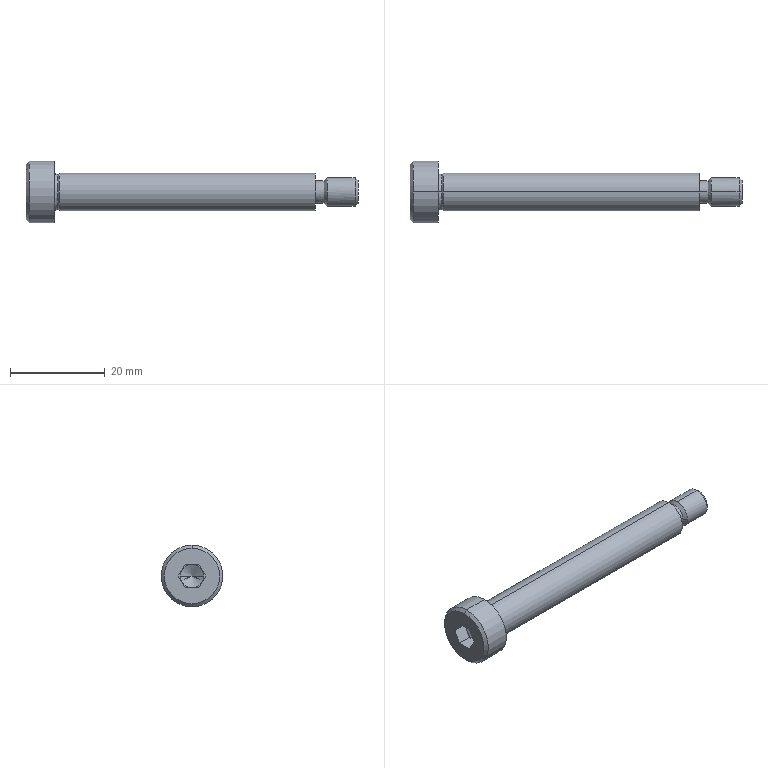Part | SolidWorks | features BaseBody 1 | 1 solid | 36 faces | box 70 x 13 x 13 mm | volume 3701 mm3 | plane 16 | cone 10 | cylinder 8 | spline 2 | commonest cylinder face diameters 4.7 x2 6 x2 8 x2 13 x2
STEP:
#1=CARTESIAN_POINT('',(0.,0.,4.35));
#2=VERTEX_POINT('',#1);
#3=CARTESIAN_POINT('',(0.,0.,-4.35));
#4=VERTEX_POINT('',#3);
#5=CARTESIAN_POINT('',(0.,0.,4.35));
#6=CARTESIAN_POINT('',(0.,0.2768,4.35));
#7=CARTESIAN_POINT('',(0.,0.6845,4.312));
#8=CARTESIAN_POINT('',(0.,1.147,4.2));
#9=CARTESIAN_POINT('',(0.,1.375,4.128));
#10=CARTESIAN_POINT('',(0.,1.472,4.093));
#11=CARTESIAN_POINT('',(0.,1.537,4.07));
#12=CARTESIAN_POINT('',(0.,1.567,4.058));
#13=CARTESIAN_POINT('',(0.,1.738,3.99));
#14=CARTESIAN_POINT('',(0.,1.938,3.899));
#15=CARTESIAN_POINT('',(0.,2.13,3.793));
#16=CARTESIAN_POINT('',(0.,2.257,3.72));
#17=CARTESIAN_POINT('',(0.,2.317,3.682));
#18=CARTESIAN_POINT('',(0.,2.632,3.476));
#19=CARTESIAN_POINT('',(0.,2.863,3.289));
#20=CARTESIAN_POINT('',(0.,3.182,2.97));
#21=CARTESIAN_POINT('',(0.,3.333,2.803));
#22=CARTESIAN_POINT('',(0.,3.469,2.625));
#23=CARTESIAN_POINT('',(0.,3.557,2.505));
#24=CARTESIAN_POINT('',(0.,3.601,2.442));
#25=CARTESIAN_POINT('',(0.,3.721,2.257));
#26=CARTESIAN_POINT('',(0.,3.832,2.067));
#27=CARTESIAN_POINT('',(0.,3.944,1.837));
#28=CARTESIAN_POINT('',(0.,3.988,1.737));
#29=CARTESIAN_POINT('',(0.,4.017,1.669));
#30=CARTESIAN_POINT('',(0.,4.032,1.633));
#31=CARTESIAN_POINT('',(0.,4.248,1.087));
#32=CARTESIAN_POINT('',(0.,4.35,0.5535));
#33=CARTESIAN_POINT('',(0.,4.35,-0.2768));
#34=CARTESIAN_POINT('',(0.,4.312,-0.6845));
#35=CARTESIAN_POINT('',(0.,4.2,-1.147));
#36=CARTESIAN_POINT('',(0.,4.128,-1.375));
#37=CARTESIAN_POINT('',(0.,4.093,-1.472));
#38=CARTESIAN_POINT('',(0.,4.07,-1.537));
#39=CARTESIAN_POINT('',(0.,4.058,-1.567));
#40=CARTESIAN_POINT('',(0.,3.99,-1.738));
#41=CARTESIAN_POINT('',(0.,3.899,-1.938));
#42=CARTESIAN_POINT('',(0.,3.793,-2.13));
#43=CARTESIAN_POINT('',(0.,3.72,-2.257));
#44=CARTESIAN_POINT('',(0.,3.682,-2.317));
#45=CARTESIAN_POINT('',(0.,3.476,-2.632));
#46=CARTESIAN_POINT('',(0.,3.289,-2.863));
#47=CARTESIAN_POINT('',(0.,2.97,-3.182));
#48=CARTESIAN_POINT('',(0.,2.803,-3.333));
#49=CARTESIAN_POINT('',(0.,2.625,-3.469));
#50=CARTESIAN_POINT('',(0.,2.505,-3.557));
#51=CARTESIAN_POINT('',(0.,2.442,-3.601));
#52=CARTESIAN_POINT('',(0.,2.257,-3.721));
#53=CARTESIAN_POINT('',(0.,2.067,-3.832));
#54=CARTESIAN_POINT('',(0.,1.837,-3.944));
#55=CARTESIAN_POINT('',(0.,1.737,-3.988));
#56=CARTESIAN_POINT('',(0.,1.669,-4.017));
#57=CARTESIAN_POINT('',(0.,1.633,-4.032));
#58=CARTESIAN_POINT('',(0.,1.087,-4.248));
#59=CARTESIAN_POINT('',(0.,0.553,-4.35));
#60=CARTESIAN_POINT('',(0.,0.,-4.35));
#61=B_SPLINE_CURVE_WITH_KNOTS('',3,(#5,#6,#7,#8,#9,#10,#11,#12,#13,#14,#15,#16,#17,#18,#19,#20,#21,#22,#23,#24,#25,#26,#27,#28,#29,#30,#31,#32,#33,#34,#35,#36,#37,#38,#39,#40,#41,#42,#43,#44,#45,#46,#47,#48,#49,#50,#51,#52,#53,#54,#55,#56,#57,#58,#59,#60),.UNSPECIFIED.,.F.,.F.,(4,1,1,1,2,2,1,2,2,2,1,2,2,1,1,2,2,2,1,1,1,2,2,1,2,2,2,1,2,2,1,1,2,2,4),(0.5,0.5313,0.5469,0.5547,0.5586,0.5625,0.5781,0.5859,0.5938,0.625,0.6406,0.6484,0.6563,0.6719,0.6797,0.6836,0.6875,0.75,0.7813,0.7969,0.8047,0.8086,0.8125,0.8281,0.8359,0.8438,0.875,0.8906,0.8984,0.9063,0.9219,0.9297,0.9336,0.9375,1.),.UNSPECIFIED.);
#62=EDGE_CURVE('',#2,#4,#61,.T.);
#63=ORIENTED_EDGE('',*,*,#62,.F.);
#64=CARTESIAN_POINT('',(0.7,0.,3.7));
#65=VERTEX_POINT('',#64);
#66=CARTESIAN_POINT('',(0.6306,0.,4.327));
#67=DIRECTION('',(0.,-1.,0.));
#68=DIRECTION('',(0.,0.,1.));
#69=AXIS2_PLACEMENT_3D('',#66,#67,#68);
#70=CIRCLE('',#69,0.631);
#71=EDGE_CURVE('',#2,#65,#70,.T.);
#72=ORIENTED_EDGE('',*,*,#71,.T.);
#73=CARTESIAN_POINT('',(0.7,0.,-3.7));
#74=VERTEX_POINT('',#73);
#75=CARTESIAN_POINT('',(0.7,0.,0.));
#76=DIRECTION('',(1.,0.,0.));
#77=DIRECTION('',(0.,0.,-1.));
#78=AXIS2_PLACEMENT_3D('',#75,#76,#77);
#79=CIRCLE('',#78,3.7);
#80=EDGE_CURVE('',#74,#65,#79,.T.);
#81=ORIENTED_EDGE('',*,*,#80,.F.);
#82=CARTESIAN_POINT('',(0.6306,0.,-4.327));
#83=DIRECTION('',(0.,1.,0.));
#84=DIRECTION('',(0.,0.,-1.));
#85=AXIS2_PLACEMENT_3D('',#82,#83,#84);
#86=CIRCLE('',#85,0.631);
#87=EDGE_CURVE('',#4,#74,#86,.T.);
#88=ORIENTED_EDGE('',*,*,#87,.F.);
#89=EDGE_LOOP('',(#63,#72,#81,#88));
#90=FACE_OUTER_BOUND('',#89,.T.);
#91=CARTESIAN_POINT('',(0.,0.,-4.35));
#92=CARTESIAN_POINT('',(0.,8.7,-4.35));
#93=CARTESIAN_POINT('',(0.,8.7,4.35));
#94=CARTESIAN_POINT('',(0.,0.,4.35));
#95=CARTESIAN_POINT('',(-0.01498,0.,-3.936));
#96=CARTESIAN_POINT('',(-0.01498,7.872,-3.936));
#97=CARTESIAN_POINT('',(-0.01498,7.872,3.936));
#98=CARTESIAN_POINT('',(-0.01498,0.,3.936));
#99=CARTESIAN_POINT('',(0.2884,0.,-3.654));
#100=CARTESIAN_POINT('',(0.2884,7.309,-3.654));
#101=CARTESIAN_POINT('',(0.2884,7.309,3.654));
#102=CARTESIAN_POINT('',(0.2884,0.,3.654));
#103=CARTESIAN_POINT('',(0.7,0.,-3.7));
#104=CARTESIAN_POINT('',(0.7,7.4,-3.7));
#105=CARTESIAN_POINT('',(0.7,7.4,3.7));
#106=CARTESIAN_POINT('',(0.7,0.,3.7));
#107=(BOUNDED_SURFACE()B_SPLINE_SURFACE(3,3,((#91,#92,#93,#94),(#95,#96,#97,#98),(#99,#100,#101,#102),(#103,#104,#105,#106)),.UNSPECIFIED.,.F.,.F.,.T.)B_SPLINE_SURFACE_WITH_KNOTS((4,4),(4,4),(0.,1.),(0.,1.),.UNSPECIFIED.)GEOMETRIC_REPRESENTATION_ITEM()RATIONAL_B_SPLINE_SURFACE(((1.,0.3333,0.3333,1.),(0.769,0.2563,0.2563,0.769),(0.769,0.2563,0.2563,0.769),(1.,0.3333,0.3333,1.)))REPRESENTATION_ITEM('')SURFACE());
#108=ADVANCED_FACE('',(#90),#107,.F.);
#109=CARTESIAN_POINT('',(55.,0.,4.));
#110=VERTEX_POINT('',#109);
#111=CARTESIAN_POINT('',(55.,0.,-4.));
#112=VERTEX_POINT('',#111);
#113=CARTESIAN_POINT('',(55.,0.,0.));
#114=DIRECTION('',(-1.,0.,0.));
#115=DIRECTION('',(0.,0.,1.));
#116=AXIS2_PLACEMENT_3D('',#113,#114,#115);
#117=CIRCLE('',#116,4.);
#118=EDGE_CURVE('',#110,#112,#117,.T.);
#119=ORIENTED_EDGE('',*,*,#118,.T.);
#120=CARTESIAN_POINT('',(1.,0.,-4.));
#121=VERTEX_POINT('',#120);
#122=CARTESIAN_POINT('',(64.,0.,-4.));
#123=DIRECTION('',(-1.,0.,0.));
#124=VECTOR('',#123,1000.);
#125=LINE('',#122,#124);
#126=EDGE_CURVE('',#112,#121,#125,.T.);
#127=ORIENTED_EDGE('',*,*,#126,.T.);
#128=CARTESIAN_POINT('',(1.,0.,4.));
#129=VERTEX_POINT('',#128);
#130=CARTESIAN_POINT('',(1.,0.,0.));
#131=DIRECTION('',(1.,0.,0.));
#132=DIRECTION('',(0.,0.,1.));
#133=AXIS2_PLACEMENT_3D('',#130,#131,#132);
#134=CIRCLE('',#133,4.);
#135=EDGE_CURVE('',#121,#129,#134,.T.);
#136=ORIENTED_EDGE('',*,*,#135,.T.);
#137=CARTESIAN_POINT('',(64.,0.,4.));
#138=DIRECTION('',(-1.,0.,0.));
#139=VECTOR('',#138,1000.);
#140=LINE('',#137,#139);
#141=EDGE_CURVE('',#110,#129,#140,.T.);
#142=ORIENTED_EDGE('',*,*,#141,.F.);
#143=EDGE_LOOP('',(#119,#127,#136,#142));
#144=FACE_OUTER_BOUND('',#143,.T.);
#145=CARTESIAN_POINT('',(64.,0.,0.));
#146=DIRECTION('',(-1.,0.,0.));
#147=DIRECTION('',(0.,0.,1.));
#148=AXIS2_PLACEMENT_3D('',#145,#146,#147);
#149=CYLINDRICAL_SURFACE('',#148,4.);
#150=ADVANCED_FACE('',(#144),#149,.T.);
#151=ORIENTED_EDGE('',*,*,#80,.T.);
#152=CARTESIAN_POINT('',(1.,0.,4.));
#153=DIRECTION('',(0.7071,0.,0.7071));
#154=VECTOR('',#153,1000.);
#155=LINE('',#152,#154);
#156=EDGE_CURVE('',#65,#129,#155,.T.);
#157=ORIENTED_EDGE('',*,*,#156,.T.);
#158=ORIENTED_EDGE('',*,*,#135,.F.);
#159=CARTESIAN_POINT('',(1.,0.,-4.));
#160=DIRECTION('',(0.7071,0.,-0.7071));
#161=VECTOR('',#160,1000.);
#162=LINE('',#159,#161);
#163=EDGE_CURVE('',#74,#121,#162,.T.);
#164=ORIENTED_EDGE('',*,*,#163,.F.);
#165=EDGE_LOOP('',(#151,#157,#158,#164));
#166=FACE_OUTER_BOUND('',#165,.T.);
#167=CARTESIAN_POINT('',(1.,0.,0.));
#168=DIRECTION('',(1.,0.,0.));
#169=DIRECTION('',(0.,0.,-1.));
#170=AXIS2_PLACEMENT_3D('',#167,#168,#169);
#171=CONICAL_SURFACE('',#170,4.,0.7854);
#172=ADVANCED_FACE('',(#166),#171,.T.);
#173=CARTESIAN_POINT('',(56.85,2.35,0.));
#174=VERTEX_POINT('',#173);
#175=CARTESIAN_POINT('',(56.85,0.,-2.35));
#176=VERTEX_POINT('',#175);
#177=CARTESIAN_POINT('',(56.85,0.,0.));
#178=DIRECTION('',(-1.,0.,0.));
#179=DIRECTION('',(0.,0.,1.));
#180=AXIS2_PLACEMENT_3D('',#177,#178,#179);
#181=CIRCLE('',#180,2.35);
#182=EDGE_CURVE('',#174,#176,#181,.T.);
#183=ORIENTED_EDGE('',*,*,#182,.T.);
#184=CARTESIAN_POINT('',(55.,0.,-2.35));
#185=VERTEX_POINT('',#184);
#186=CARTESIAN_POINT('',(64.,0.,-2.35));
#187=DIRECTION('',(-1.,0.,0.));
#188=VECTOR('',#187,1000.);
#189=LINE('',#186,#188);
#190=EDGE_CURVE('',#176,#185,#189,.T.);
#191=ORIENTED_EDGE('',*,*,#190,.T.);
#192=CARTESIAN_POINT('',(55.,0.,2.35));
#193=VERTEX_POINT('',#192);
#194=CARTESIAN_POINT('',(55.,0.,0.));
#195=DIRECTION('',(1.,0.,0.));
#196=DIRECTION('',(0.,0.,1.));
#197=AXIS2_PLACEMENT_3D('',#194,#195,#196);
#198=CIRCLE('',#197,2.35);
#199=EDGE_CURVE('',#185,#193,#198,.T.);
#200=ORIENTED_EDGE('',*,*,#199,.T.);
#201=CARTESIAN_POINT('',(56.85,0.,2.35));
#202=VERTEX_POINT('',#201);
#203=CARTESIAN_POINT('',(64.,0.,2.35));
#204=DIRECTION('',(-1.,0.,0.));
#205=VECTOR('',#204,1000.);
#206=LINE('',#203,#205);
#207=EDGE_CURVE('',#202,#193,#206,.T.);
#208=ORIENTED_EDGE('',*,*,#207,.F.);
#209=CARTESIAN_POINT('',(56.85,0.,0.));
#210=DIRECTION('',(-1.,0.,0.));
#211=DIRECTION('',(0.,0.,1.));
#212=AXIS2_PLACEMENT_3D('',#209,#210,#211);
#213=CIRCLE('',#212,2.35);
#214=EDGE_CURVE('',#202,#174,#213,.T.);
#215=ORIENTED_EDGE('',*,*,#214,.T.);
#216=EDGE_LOOP('',(#183,#191,#200,#208,#215));
#217=FACE_OUTER_BOUND('',#216,.T.);
#218=CARTESIAN_POINT('',(64.,0.,0.));
#219=DIRECTION('',(-1.,0.,0.));
#220=DIRECTION('',(0.,0.,1.));
#221=AXIS2_PLACEMENT_3D('',#218,#219,#220);
#222=CYLINDRICAL_SURFACE('',#221,2.35);
#223=ADVANCED_FACE('',(#217),#222,.T.);
#224=CARTESIAN_POINT('',(56.85,-2.35,0.));
#225=VERTEX_POINT('',#224);
#226=CARTESIAN_POINT('',(56.85,0.,0.));
#227=DIRECTION('',(-1.,0.,0.));
#228=DIRECTION('',(0.,0.,1.));
#229=AXIS2_PLACEMENT_3D('',#226,#227,#228);
#230=CIRCLE('',#229,2.35);
#231=EDGE_CURVE('',#225,#202,#230,.T.);
#232=ORIENTED_EDGE('',*,*,#231,.F.);
#233=CARTESIAN_POINT('',(57.5,-3.,0.));
#234=VERTEX_POINT('',#233);
#235=CARTESIAN_POINT('',(57.5,-3.,0.));
#236=DIRECTION('',(0.7071,-0.7071,0.));
#237=VECTOR('',#236,1000.);
#238=LINE('',#235,#237);
#239=EDGE_CURVE('',#225,#234,#238,.T.);
#240=ORIENTED_EDGE('',*,*,#239,.T.);
#241=CARTESIAN_POINT('',(57.5,0.,3.));
#242=VERTEX_POINT('',#241);
#243=CARTESIAN_POINT('',(57.5,0.,0.));
#244=DIRECTION('',(-1.,0.,0.));
#245=DIRECTION('',(0.,0.,-1.));
#246=AXIS2_PLACEMENT_3D('',#243,#244,#245);
#247=CIRCLE('',#246,3.);
#248=EDGE_CURVE('',#234,#242,#247,.T.);
#249=ORIENTED_EDGE('',*,*,#248,.T.);
#250=CARTESIAN_POINT('',(57.5,3.,0.));
#251=VERTEX_POINT('',#250);
#252=CARTESIAN_POINT('',(57.5,0.,0.));
#253=DIRECTION('',(-1.,0.,0.));
#254=DIRECTION('',(0.,0.,-1.));
#255=AXIS2_PLACEMENT_3D('',#252,#253,#254);
#256=CIRCLE('',#255,3.);
#257=EDGE_CURVE('',#242,#251,#256,.T.);
#258=ORIENTED_EDGE('',*,*,#257,.T.);
#259=CARTESIAN_POINT('',(57.5,3.,0.));
#260=DIRECTION('',(0.7071,0.7071,0.));
#261=VECTOR('',#260,1000.);
#262=LINE('',#259,#261);
#263=EDGE_CURVE('',#174,#251,#262,.T.);
#264=ORIENTED_EDGE('',*,*,#263,.F.);
#265=ORIENTED_EDGE('',*,*,#214,.F.);
#266=EDGE_LOOP('',(#232,#240,#249,#258,#264,#265));
#267=FACE_OUTER_BOUND('',#266,.T.);
#268=CARTESIAN_POINT('',(57.5,0.,0.));
#269=DIRECTION('',(1.,0.,0.));
#270=DIRECTION('',(0.,1.,0.));
#271=AXIS2_PLACEMENT_3D('',#268,#269,#270);
#272=CONICAL_SURFACE('',#271,3.,0.7854);
#273=ADVANCED_FACE('',(#267),#272,.T.);
#274=CARTESIAN_POINT('',(0.,0.,6.5));
#275=VERTEX_POINT('',#274);
#276=CARTESIAN_POINT('',(0.,0.,-6.5));
#277=VERTEX_POINT('',#276);
#278=CARTESIAN_POINT('',(0.,0.,0.));
#279=DIRECTION('',(-1.,0.,0.));
#280=DIRECTION('',(0.,0.,1.));
#281=AXIS2_PLACEMENT_3D('',#278,#279,#280);
#282=CIRCLE('',#281,6.5);
#283=EDGE_CURVE('',#275,#277,#282,.T.);
#284=ORIENTED_EDGE('',*,*,#283,.T.);
#285=CARTESIAN_POINT('',(-5.35,0.,-6.5));
#286=VERTEX_POINT('',#285);
#287=CARTESIAN_POINT('',(64.,0.,-6.5));
#288=DIRECTION('',(-1.,0.,0.));
#289=VECTOR('',#288,1000.);
#290=LINE('',#287,#289);
#291=EDGE_CURVE('',#277,#286,#290,.T.);
#292=ORIENTED_EDGE('',*,*,#291,.T.);
#293=CARTESIAN_POINT('',(-5.35,0.,6.5));
#294=VERTEX_POINT('',#293);
#295=CARTESIAN_POINT('',(-5.35,0.,0.));
#296=DIRECTION('',(1.,0.,0.));
#297=DIRECTION('',(0.,0.,1.));
#298=AXIS2_PLACEMENT_3D('',#295,#296,#297);
#299=CIRCLE('',#298,6.5);
#300=EDGE_CURVE('',#286,#294,#299,.T.);
#301=ORIENTED_EDGE('',*,*,#300,.T.);
#302=CARTESIAN_POINT('',(64.,0.,6.5));
#303=DIRECTION('',(-1.,0.,0.));
#304=VECTOR('',#303,1000.);
#305=LINE('',#302,#304);
#306=EDGE_CURVE('',#275,#294,#305,.T.);
#307=ORIENTED_EDGE('',*,*,#306,.F.);
#308=EDGE_LOOP('',(#284,#292,#301,#307));
#309=FACE_OUTER_BOUND('',#308,.T.);
#310=CARTESIAN_POINT('',(64.,0.,0.));
#311=DIRECTION('',(-1.,0.,0.));
#312=DIRECTION('',(0.,0.,1.));
#313=AXIS2_PLACEMENT_3D('',#310,#311,#312);
#314=CYLINDRICAL_SURFACE('',#313,6.5);
#315=ADVANCED_FACE('',(#309),#314,.T.);
#316=CARTESIAN_POINT('',(63.386,0.,3.));
#317=VERTEX_POINT('',#316);
#318=CARTESIAN_POINT('',(63.386,0.,-3.));
#319=VERTEX_POINT('',#318);
#320=CARTESIAN_POINT('',(63.386,0.,0.));
#321=DIRECTION('',(-1.,0.,0.));
#322=DIRECTION('',(0.,0.,1.));
#323=AXIS2_PLACEMENT_3D('',#320,#321,#322);
#324=CIRCLE('',#323,3.);
#325=EDGE_CURVE('',#317,#319,#324,.T.);
#326=ORIENTED_EDGE('',*,*,#325,.T.);
#327=CARTESIAN_POINT('',(57.5,0.,-3.));
#328=VERTEX_POINT('',#327);
#329=CARTESIAN_POINT('',(64.,0.,-3.));
#330=DIRECTION('',(-1.,0.,0.));
#331=VECTOR('',#330,1000.);
#332=LINE('',#329,#331);
#333=EDGE_CURVE('',#319,#328,#332,.T.);
#334=ORIENTED_EDGE('',*,*,#333,.T.);
#335=CARTESIAN_POINT('',(57.5,0.,0.));
#336=DIRECTION('',(-1.,0.,0.));
#337=DIRECTION('',(0.,0.,-1.));
#338=AXIS2_PLACEMENT_3D('',#335,#336,#337);
#339=CIRCLE('',#338,3.);
#340=EDGE_CURVE('',#251,#328,#339,.T.);
#341=ORIENTED_EDGE('',*,*,#340,.F.);
#342=ORIENTED_EDGE('',*,*,#257,.F.);
#343=CARTESIAN_POINT('',(64.,0.,3.));
#344=DIRECTION('',(-1.,0.,0.));
#345=VECTOR('',#344,1000.);
#346=LINE('',#343,#345);
#347=EDGE_CURVE('',#317,#242,#346,.T.);
#348=ORIENTED_EDGE('',*,*,#347,.F.);
#349=EDGE_LOOP('',(#326,#334,#341,#342,#348));
#350=FACE_OUTER_BOUND('',#349,.T.);
#351=CARTESIAN_POINT('',(64.,0.,0.));
#352=DIRECTION('',(-1.,0.,0.));
#353=DIRECTION('',(0.,0.,1.));
#354=AXIS2_PLACEMENT_3D('',#351,#352,#353);
#355=CYLINDRICAL_SURFACE('',#354,3.);
#356=ADVANCED_FACE('',(#350),#355,.T.);
#357=CARTESIAN_POINT('',(-6.,0.,-5.85));
#358=VERTEX_POINT('',#357);
#359=CARTESIAN_POINT('',(-6.,0.,5.85));
#360=VERTEX_POINT('',#359);
#361=CARTESIAN_POINT('',(-6.,0.,0.));
#362=DIRECTION('',(1.,0.,0.));
#363=DIRECTION('',(0.,0.,-1.));
#364=AXIS2_PLACEMENT_3D('',#361,#362,#363);
#365=CIRCLE('',#364,5.85);
#366=EDGE_CURVE('',#358,#360,#365,.T.);
#367=ORIENTED_EDGE('',*,*,#366,.T.);
#368=CARTESIAN_POINT('',(-5.35,0.,6.5));
#369=DIRECTION('',(0.7071,0.,0.7071));
#370=VECTOR('',#369,1000.);
#371=LINE('',#368,#370);
#372=EDGE_CURVE('',#360,#294,#371,.T.);
#373=ORIENTED_EDGE('',*,*,#372,.T.);
#374=ORIENTED_EDGE('',*,*,#300,.F.);
#375=CARTESIAN_POINT('',(-5.35,0.,-6.5));
#376=DIRECTION('',(0.7071,0.,-0.7071));
#377=VECTOR('',#376,1000.);
#378=LINE('',#375,#377);
#379=EDGE_CURVE('',#358,#286,#378,.T.);
#380=ORIENTED_EDGE('',*,*,#379,.F.);
#381=EDGE_LOOP('',(#367,#373,#374,#380));
#382=FACE_OUTER_BOUND('',#381,.T.);
#383=CARTESIAN_POINT('',(-5.35,0.,0.));
#384=DIRECTION('',(1.,0.,0.));
#385=DIRECTION('',(0.,0.,-1.));
#386=AXIS2_PLACEMENT_3D('',#383,#384,#385);
#387=CONICAL_SURFACE('',#386,6.5,0.7854);
#388=ADVANCED_FACE('',(#382),#387,.T.);
#389=CARTESIAN_POINT('',(64.,0.,2.386));
#390=VERTEX_POINT('',#389);
#391=CARTESIAN_POINT('',(64.,0.,-2.386));
#392=VERTEX_POINT('',#391);
#393=CARTESIAN_POINT('',(64.,0.,0.));
#394=DIRECTION('',(-1.,0.,0.));
#395=DIRECTION('',(0.,0.,1.));
#396=AXIS2_PLACEMENT_3D('',#393,#394,#395);
#397=CIRCLE('',#396,2.386);
#398=EDGE_CURVE('',#390,#392,#397,.T.);
#399=ORIENTED_EDGE('',*,*,#398,.T.);
#400=CARTESIAN_POINT('',(63.387,0.,-3.));
#401=DIRECTION('',(-0.7071,0.,-0.7071));
#402=VECTOR('',#401,1000.);
#403=LINE('',#400,#402);
#404=EDGE_CURVE('',#392,#319,#403,.T.);
#405=ORIENTED_EDGE('',*,*,#404,.T.);
#406=ORIENTED_EDGE('',*,*,#325,.F.);
#407=CARTESIAN_POINT('',(63.387,0.,3.));
#408=DIRECTION('',(-0.7071,0.,0.7071));
#409=VECTOR('',#408,1000.);
#410=LINE('',#407,#409);
#411=EDGE_CURVE('',#390,#317,#410,.T.);
#412=ORIENTED_EDGE('',*,*,#411,.F.);
#413=EDGE_LOOP('',(#399,#405,#406,#412));
#414=FACE_OUTER_BOUND('',#413,.T.);
#415=CARTESIAN_POINT('',(63.387,0.,0.));
#416=DIRECTION('',(-1.,0.,0.));
#417=DIRECTION('',(0.,0.,1.));
#418=AXIS2_PLACEMENT_3D('',#415,#416,#417);
#419=CONICAL_SURFACE('',#418,3.,0.7854);
#420=ADVANCED_FACE('',(#414),#419,.T.);
#421=CARTESIAN_POINT('',(-1.557,0.,0.));
#422=VERTEX_POINT('',#421);
#423=CARTESIAN_POINT('',(-3.,-2.5,0.));
#424=VERTEX_POINT('',#423);
#425=CARTESIAN_POINT('',(-3.,-2.5,0.));
#426=DIRECTION('',(-0.5,-0.866,0.));
#427=VECTOR('',#426,1000.);
#428=LINE('',#425,#427);
#429=EDGE_CURVE('',#422,#424,#428,.T.);
#430=ORIENTED_EDGE('',*,*,#429,.F.);
#431=CARTESIAN_POINT('',(-3.,2.5,0.));
#432=VERTEX_POINT('',#431);
#433=CARTESIAN_POINT('',(-3.,2.5,0.));
#434=DIRECTION('',(-0.5,0.866,0.));
#435=VECTOR('',#434,1000.);
#436=LINE('',#433,#435);
#437=EDGE_CURVE('',#422,#432,#436,.T.);
#438=ORIENTED_EDGE('',*,*,#437,.T.);
#439=CARTESIAN_POINT('',(-3.,2.165,-1.25));
#440=VERTEX_POINT('',#439);
#441=CARTESIAN_POINT('',(-3.,0.,0.));
#442=DIRECTION('',(1.,0.,0.));
#443=DIRECTION('',(0.,-1.,0.));
#444=AXIS2_PLACEMENT_3D('',#441,#442,#443);
#445=CIRCLE('',#444,2.5);
#446=EDGE_CURVE('',#440,#432,#445,.T.);
#447=ORIENTED_EDGE('',*,*,#446,.F.);
#448=CARTESIAN_POINT('',(-3.,0.,-2.5));
#449=VERTEX_POINT('',#448);
#450=CARTESIAN_POINT('',(-3.,0.,0.));
#451=DIRECTION('',(1.,0.,0.));
#452=DIRECTION('',(0.,-1.,0.));
#453=AXIS2_PLACEMENT_3D('',#450,#451,#452);
#454=CIRCLE('',#453,2.5);
#455=EDGE_CURVE('',#449,#440,#454,.T.);
#456=ORIENTED_EDGE('',*,*,#455,.F.);
#457=CARTESIAN_POINT('',(-3.,-2.165,-1.25));
#458=VERTEX_POINT('',#457);
#459=CARTESIAN_POINT('',(-3.,0.,0.));
#460=DIRECTION('',(1.,0.,0.));
#461=DIRECTION('',(0.,-1.,0.));
#462=AXIS2_PLACEMENT_3D('',#459,#460,#461);
#463=CIRCLE('',#462,2.5);
#464=EDGE_CURVE('',#458,#449,#463,.T.);
#465=ORIENTED_EDGE('',*,*,#464,.F.);
#466=CARTESIAN_POINT('',(-3.,0.,0.));
#467=DIRECTION('',(1.,0.,0.));
#468=DIRECTION('',(0.,-1.,0.));
#469=AXIS2_PLACEMENT_3D('',#466,#467,#468);
#470=CIRCLE('',#469,2.5);
#471=EDGE_CURVE('',#424,#458,#470,.T.);
#472=ORIENTED_EDGE('',*,*,#471,.F.);
#473=EDGE_LOOP('',(#430,#438,#447,#456,#465,#472));
#474=FACE_OUTER_BOUND('',#473,.T.);
#475=CARTESIAN_POINT('',(-3.,0.,0.));
#476=DIRECTION('',(-1.,0.,0.));
#477=DIRECTION('',(0.,-1.,0.));
#478=AXIS2_PLACEMENT_3D('',#475,#476,#477);
#479=CONICAL_SURFACE('',#478,2.5,1.047);
#480=ADVANCED_FACE('',(#474),#479,.F.);
#481=ORIENTED_EDGE('',*,*,#126,.F.);
#482=CARTESIAN_POINT('',(55.,0.,0.));
#483=DIRECTION('',(-1.,0.,0.));
#484=DIRECTION('',(0.,0.,1.));
#485=AXIS2_PLACEMENT_3D('',#482,#483,#484);
#486=CIRCLE('',#485,4.);
#487=EDGE_CURVE('',#112,#110,#486,.T.);
#488=ORIENTED_EDGE('',*,*,#487,.T.);
#489=ORIENTED_EDGE('',*,*,#141,.T.);
#490=CARTESIAN_POINT('',(1.,0.,0.));
#491=DIRECTION('',(1.,0.,0.));
#492=DIRECTION('',(0.,0.,1.));
#493=AXIS2_PLACEMENT_3D('',#490,#491,#492);
#494=CIRCLE('',#493,4.);
#495=EDGE_CURVE('',#129,#121,#494,.T.);
#496=ORIENTED_EDGE('',*,*,#495,.T.);
#497=EDGE_LOOP('',(#481,#488,#489,#496));
#498=FACE_OUTER_BOUND('',#497,.T.);
#499=CARTESIAN_POINT('',(64.,0.,0.));
#500=DIRECTION('',(-1.,0.,0.));
#501=DIRECTION('',(0.,0.,1.));
#502=AXIS2_PLACEMENT_3D('',#499,#500,#501);
#503=CYLINDRICAL_SURFACE('',#502,4.);
#504=ADVANCED_FACE('',(#498),#503,.T.);
#505=ORIENTED_EDGE('',*,*,#156,.F.);
#506=CARTESIAN_POINT('',(0.7,0.,0.));
#507=DIRECTION('',(1.,0.,0.));
#508=DIRECTION('',(0.,0.,-1.));
#509=AXIS2_PLACEMENT_3D('',#506,#507,#508);
#510=CIRCLE('',#509,3.7);
#511=EDGE_CURVE('',#65,#74,#510,.T.);
#512=ORIENTED_EDGE('',*,*,#511,.T.);
#513=ORIENTED_EDGE('',*,*,#163,.T.);
#514=ORIENTED_EDGE('',*,*,#495,.F.);
#515=EDGE_LOOP('',(#505,#512,#513,#514));
#516=FACE_OUTER_BOUND('',#515,.T.);
#517=CARTESIAN_POINT('',(1.,0.,0.));
#518=DIRECTION('',(1.,0.,0.));
#519=DIRECTION('',(0.,0.,-1.));
#520=AXIS2_PLACEMENT_3D('',#517,#518,#519);
#521=CONICAL_SURFACE('',#520,4.,0.7854);
#522=ADVANCED_FACE('',(#516),#521,.T.);
#523=ORIENTED_EDGE('',*,*,#118,.F.);
#524=ORIENTED_EDGE('',*,*,#487,.F.);
#525=EDGE_LOOP('',(#523,#524));
#526=FACE_OUTER_BOUND('',#525,.T.);
#527=CARTESIAN_POINT('',(55.,0.,0.));
#528=DIRECTION('',(1.,0.,0.));
#529=DIRECTION('',(0.,0.,1.));
#530=AXIS2_PLACEMENT_3D('',#527,#528,#529);
#531=CIRCLE('',#530,2.35);
#532=EDGE_CURVE('',#193,#185,#531,.T.);
#533=ORIENTED_EDGE('',*,*,#532,.F.);
#534=ORIENTED_EDGE('',*,*,#199,.F.);
#535=EDGE_LOOP('',(#533,#534));
#536=FACE_BOUND('',#535,.T.);
#537=CARTESIAN_POINT('',(55.,4.,0.));
#538=DIRECTION('',(-1.,0.,0.));
#539=DIRECTION('',(0.,0.,1.));
#540=AXIS2_PLACEMENT_3D('',#537,#538,#539);
#541=PLANE('',#540);
#542=ADVANCED_FACE('',(#526,#536),#541,.F.);
#543=ORIENTED_EDGE('',*,*,#71,.F.);
#544=CARTESIAN_POINT('',(0.,0.,-4.35));
#545=CARTESIAN_POINT('',(0.,-0.2767,-4.35));
#546=CARTESIAN_POINT('',(0.,-0.6843,-4.312));
#547=CARTESIAN_POINT('',(0.,-1.147,-4.2));
#548=CARTESIAN_POINT('',(0.,-1.375,-4.128));
#549=CARTESIAN_POINT('',(0.,-1.472,-4.093));
#550=CARTESIAN_POINT('',(0.,-1.537,-4.07));
#551=CARTESIAN_POINT('',(0.,-1.567,-4.058));
#552=CARTESIAN_POINT('',(0.,-1.738,-3.99));
#553=CARTESIAN_POINT('',(0.,-1.938,-3.899));
#554=CARTESIAN_POINT('',(0.,-2.13,-3.793));
#555=CARTESIAN_POINT('',(0.,-2.257,-3.72));
#556=CARTESIAN_POINT('',(0.,-2.317,-3.682));
#557=CARTESIAN_POINT('',(0.,-2.632,-3.476));
#558=CARTESIAN_POINT('',(0.,-2.863,-3.289));
#559=CARTESIAN_POINT('',(0.,-3.182,-2.97));
#560=CARTESIAN_POINT('',(0.,-3.333,-2.803));
#561=CARTESIAN_POINT('',(0.,-3.469,-2.625));
#562=CARTESIAN_POINT('',(0.,-3.557,-2.505));
#563=CARTESIAN_POINT('',(0.,-3.601,-2.442));
#564=CARTESIAN_POINT('',(0.,-3.721,-2.257));
#565=CARTESIAN_POINT('',(0.,-3.832,-2.067));
#566=CARTESIAN_POINT('',(0.,-3.944,-1.837));
#567=CARTESIAN_POINT('',(0.,-3.988,-1.737));
#568=CARTESIAN_POINT('',(0.,-4.017,-1.669));
#569=CARTESIAN_POINT('',(0.,-4.032,-1.633));
#570=CARTESIAN_POINT('',(0.,-4.248,-1.087));
#571=CARTESIAN_POINT('',(0.,-4.35,-0.5535));
#572=CARTESIAN_POINT('',(0.,-4.35,0.2768));
#573=CARTESIAN_POINT('',(0.,-4.312,0.6845));
#574=CARTESIAN_POINT('',(0.,-4.2,1.147));
#575=CARTESIAN_POINT('',(0.,-4.128,1.375));
#576=CARTESIAN_POINT('',(0.,-4.093,1.472));
#577=CARTESIAN_POINT('',(0.,-4.07,1.537));
#578=CARTESIAN_POINT('',(0.,-4.058,1.567));
#579=CARTESIAN_POINT('',(0.,-3.99,1.738));
#580=CARTESIAN_POINT('',(0.,-3.899,1.938));
#581=CARTESIAN_POINT('',(0.,-3.793,2.13));
#582=CARTESIAN_POINT('',(0.,-3.72,2.257));
#583=CARTESIAN_POINT('',(0.,-3.682,2.317));
#584=CARTESIAN_POINT('',(0.,-3.476,2.632));
#585=CARTESIAN_POINT('',(0.,-3.289,2.863));
#586=CARTESIAN_POINT('',(0.,-2.97,3.182));
#587=CARTESIAN_POINT('',(0.,-2.803,3.333));
#588=CARTESIAN_POINT('',(0.,-2.625,3.469));
#589=CARTESIAN_POINT('',(0.,-2.505,3.557));
#590=CARTESIAN_POINT('',(0.,-2.442,3.601));
#591=CARTESIAN_POINT('',(0.,-2.257,3.721));
#592=CARTESIAN_POINT('',(0.,-2.067,3.832));
#593=CARTESIAN_POINT('',(0.,-1.837,3.944));
#594=CARTESIAN_POINT('',(0.,-1.737,3.988));
#595=CARTESIAN_POINT('',(0.,-1.669,4.017));
#596=CARTESIAN_POINT('',(0.,-1.633,4.032));
#597=CARTESIAN_POINT('',(0.,-1.087,4.248));
#598=CARTESIAN_POINT('',(0.,-0.5535,4.35));
#599=CARTESIAN_POINT('',(0.,0.,4.35));
#600=B_SPLINE_CURVE_WITH_KNOTS('',3,(#544,#545,#546,#547,#548,#549,#550,#551,#552,#553,#554,#555,#556,#557,#558,#559,#560,#561,#562,#563,#564,#565,#566,#567,#568,#569,#570,#571,#572,#573,#574,#575,#576,#577,#578,#579,#580,#581,#582,#583,#584,#585,#586,#587,#588,#589,#590,#591,#592,#593,#594,#595,#596,#597,#598,#599),.UNSPECIFIED.,.F.,.F.,(4,1,1,1,2,2,1,2,2,2,1,2,2,1,1,2,2,2,1,1,1,2,2,1,2,2,2,1,2,2,1,1,2,2,4),(0.,0.03125,0.04687,0.05469,0.05859,0.0625,0.07812,0.08594,0.09375,0.125,0.1406,0.1484,0.1562,0.1719,0.1797,0.1836,0.1875,0.25,0.2812,0.2969,0.3047,0.3086,0.3125,0.3281,0.3359,0.3437,0.375,0.3906,0.3984,0.4062,0.4219,0.4297,0.4336,0.4375,0.5),.UNSPECIFIED.);
#601=EDGE_CURVE('',#4,#2,#600,.T.);
#602=ORIENTED_EDGE('',*,*,#601,.F.);
#603=ORIENTED_EDGE('',*,*,#87,.T.);
#604=ORIENTED_EDGE('',*,*,#511,.F.);
#605=EDGE_LOOP('',(#543,#602,#603,#604));
#606=FACE_OUTER_BOUND('',#605,.T.);
#607=CARTESIAN_POINT('',(0.,0.,4.35));
#608=CARTESIAN_POINT('',(0.,-8.7,4.35));
#609=CARTESIAN_POINT('',(0.,-8.7,-4.35));
#610=CARTESIAN_POINT('',(0.,0.,-4.35));
#611=CARTESIAN_POINT('',(-0.01498,0.,3.936));
#612=CARTESIAN_POINT('',(-0.01498,-7.872,3.936));
#613=CARTESIAN_POINT('',(-0.01498,-7.872,-3.936));
#614=CARTESIAN_POINT('',(-0.01498,0.,-3.936));
#615=CARTESIAN_POINT('',(0.2884,0.,3.654));
#616=CARTESIAN_POINT('',(0.2884,-7.309,3.654));
#617=CARTESIAN_POINT('',(0.2884,-7.309,-3.654));
#618=CARTESIAN_POINT('',(0.2884,0.,-3.654));
#619=CARTESIAN_POINT('',(0.7,0.,3.7));
#620=CARTESIAN_POINT('',(0.7,-7.4,3.7));
#621=CARTESIAN_POINT('',(0.7,-7.4,-3.7));
#622=CARTESIAN_POINT('',(0.7,0.,-3.7));
#623=(BOUNDED_SURFACE()B_SPLINE_SURFACE(3,3,((#607,#608,#609,#610),(#611,#612,#613,#614),(#615,#616,#617,#618),(#619,#620,#621,#622)),.UNSPECIFIED.,.F.,.F.,.T.)B_SPLINE_SURFACE_WITH_KNOTS((4,4),(4,4),(0.,1.),(0.,1.),.UNSPECIFIED.)GEOMETRIC_REPRESENTATION_ITEM()RATIONAL_B_SPLINE_SURFACE(((1.,0.3333,0.3333,1.),(0.769,0.2563,0.2563,0.769),(0.769,0.2563,0.2563,0.769),(1.,0.3333,0.3333,1.)))REPRESENTATION_ITEM('')SURFACE());
#624=ADVANCED_FACE('',(#606),#623,.F.);
#625=ORIENTED_EDGE('',*,*,#190,.F.);
#626=CARTESIAN_POINT('',(56.85,0.,0.));
#627=DIRECTION('',(-1.,0.,0.));
#628=DIRECTION('',(0.,0.,1.));
#629=AXIS2_PLACEMENT_3D('',#626,#627,#628);
#630=CIRCLE('',#629,2.35);
#631=EDGE_CURVE('',#176,#225,#630,.T.);
#632=ORIENTED_EDGE('',*,*,#631,.T.);
#633=ORIENTED_EDGE('',*,*,#231,.T.);
#634=ORIENTED_EDGE('',*,*,#207,.T.);
#635=ORIENTED_EDGE('',*,*,#532,.T.);
#636=EDGE_LOOP('',(#625,#632,#633,#634,#635));
#637=FACE_OUTER_BOUND('',#636,.T.);
#638=CARTESIAN_POINT('',(64.,0.,0.));
#639=DIRECTION('',(-1.,0.,0.));
#640=DIRECTION('',(0.,0.,1.));
#641=AXIS2_PLACEMENT_3D('',#638,#639,#640);
#642=CYLINDRICAL_SURFACE('',#641,2.35);
#643=ADVANCED_FACE('',(#637),#642,.T.);
#644=ORIENTED_EDGE('',*,*,#283,.F.);
#645=CARTESIAN_POINT('',(0.,0.,0.));
#646=DIRECTION('',(-1.,0.,0.));
#647=DIRECTION('',(0.,0.,1.));
#648=AXIS2_PLACEMENT_3D('',#645,#646,#647);
#649=CIRCLE('',#648,6.5);
#650=EDGE_CURVE('',#277,#275,#649,.T.);
#651=ORIENTED_EDGE('',*,*,#650,.F.);
#652=EDGE_LOOP('',(#644,#651));
#653=FACE_OUTER_BOUND('',#652,.T.);
#654=ORIENTED_EDGE('',*,*,#601,.T.);
#655=ORIENTED_EDGE('',*,*,#62,.T.);
#656=EDGE_LOOP('',(#654,#655));
#657=FACE_BOUND('',#656,.T.);
#658=CARTESIAN_POINT('',(0.,6.5,0.));
#659=DIRECTION('',(-1.,0.,0.));
#660=DIRECTION('',(0.,0.,1.));
#661=AXIS2_PLACEMENT_3D('',#658,#659,#660);
#662=PLANE('',#661);
#663=ADVANCED_FACE('',(#653,#657),#662,.F.);
#664=ORIENTED_EDGE('',*,*,#239,.F.);
#665=ORIENTED_EDGE('',*,*,#631,.F.);
#666=ORIENTED_EDGE('',*,*,#182,.F.);
#667=ORIENTED_EDGE('',*,*,#263,.T.);
#668=ORIENTED_EDGE('',*,*,#340,.T.);
#669=CARTESIAN_POINT('',(57.5,0.,0.));
#670=DIRECTION('',(-1.,0.,0.));
#671=DIRECTION('',(0.,0.,-1.));
#672=AXIS2_PLACEMENT_3D('',#669,#670,#671);
#673=CIRCLE('',#672,3.);
#674=EDGE_CURVE('',#328,#234,#673,.T.);
#675=ORIENTED_EDGE('',*,*,#674,.T.);
#676=EDGE_LOOP('',(#664,#665,#666,#667,#668,#675));
#677=FACE_OUTER_BOUND('',#676,.T.);
#678=CARTESIAN_POINT('',(57.5,0.,0.));
#679=DIRECTION('',(1.,0.,0.));
#680=DIRECTION('',(0.,1.,0.));
#681=AXIS2_PLACEMENT_3D('',#678,#679,#680);
#682=CONICAL_SURFACE('',#681,3.,0.7854);
#683=ADVANCED_FACE('',(#677),#682,.T.);
#684=ORIENTED_EDGE('',*,*,#291,.F.);
#685=ORIENTED_EDGE('',*,*,#650,.T.);
#686=ORIENTED_EDGE('',*,*,#306,.T.);
#687=CARTESIAN_POINT('',(-5.35,0.,0.));
#688=DIRECTION('',(1.,0.,0.));
#689=DIRECTION('',(0.,0.,1.));
#690=AXIS2_PLACEMENT_3D('',#687,#688,#689);
#691=CIRCLE('',#690,6.5);
#692=EDGE_CURVE('',#294,#286,#691,.T.);
#693=ORIENTED_EDGE('',*,*,#692,.T.);
#694=EDGE_LOOP('',(#684,#685,#686,#693));
#695=FACE_OUTER_BOUND('',#694,.T.);
#696=CARTESIAN_POINT('',(64.,0.,0.));
#697=DIRECTION('',(-1.,0.,0.));
#698=DIRECTION('',(0.,0.,1.));
#699=AXIS2_PLACEMENT_3D('',#696,#697,#698);
#700=CYLINDRICAL_SURFACE('',#699,6.5);
#701=ADVANCED_FACE('',(#695),#700,.T.);
#702=ORIENTED_EDGE('',*,*,#333,.F.);
#703=CARTESIAN_POINT('',(63.386,0.,0.));
#704=DIRECTION('',(-1.,0.,0.));
#705=DIRECTION('',(0.,0.,1.));
#706=AXIS2_PLACEMENT_3D('',#703,#704,#705);
#707=CIRCLE('',#706,3.);
#708=EDGE_CURVE('',#319,#317,#707,.T.);
#709=ORIENTED_EDGE('',*,*,#708,.T.);
#710=ORIENTED_EDGE('',*,*,#347,.T.);
#711=ORIENTED_EDGE('',*,*,#248,.F.);
#712=ORIENTED_EDGE('',*,*,#674,.F.);
#713=EDGE_LOOP('',(#702,#709,#710,#711,#712));
#714=FACE_OUTER_BOUND('',#713,.T.);
#715=CARTESIAN_POINT('',(64.,0.,0.));
#716=DIRECTION('',(-1.,0.,0.));
#717=DIRECTION('',(0.,0.,1.));
#718=AXIS2_PLACEMENT_3D('',#715,#716,#717);
#719=CYLINDRICAL_SURFACE('',#718,3.);
#720=ADVANCED_FACE('',(#714),#719,.T.);
#721=ORIENTED_EDGE('',*,*,#372,.F.);
#722=CARTESIAN_POINT('',(-6.,0.,0.));
#723=DIRECTION('',(1.,0.,0.));
#724=DIRECTION('',(0.,0.,-1.));
#725=AXIS2_PLACEMENT_3D('',#722,#723,#724);
#726=CIRCLE('',#725,5.85);
#727=EDGE_CURVE('',#360,#358,#726,.T.);
#728=ORIENTED_EDGE('',*,*,#727,.T.);
#729=ORIENTED_EDGE('',*,*,#379,.T.);
#730=ORIENTED_EDGE('',*,*,#692,.F.);
#731=EDGE_LOOP('',(#721,#728,#729,#730));
#732=FACE_OUTER_BOUND('',#731,.T.);
#733=CARTESIAN_POINT('',(-5.35,0.,0.));
#734=DIRECTION('',(1.,0.,0.));
#735=DIRECTION('',(0.,0.,-1.));
#736=AXIS2_PLACEMENT_3D('',#733,#734,#735);
#737=CONICAL_SURFACE('',#736,6.5,0.7854);
#738=ADVANCED_FACE('',(#732),#737,.T.);
#739=ORIENTED_EDGE('',*,*,#404,.F.);
#740=CARTESIAN_POINT('',(64.,0.,0.));
#741=DIRECTION('',(-1.,0.,0.));
#742=DIRECTION('',(0.,0.,1.));
#743=AXIS2_PLACEMENT_3D('',#740,#741,#742);
#744=CIRCLE('',#743,2.386);
#745=EDGE_CURVE('',#392,#390,#744,.T.);
#746=ORIENTED_EDGE('',*,*,#745,.T.);
#747=ORIENTED_EDGE('',*,*,#411,.T.);
#748=ORIENTED_EDGE('',*,*,#708,.F.);
#749=EDGE_LOOP('',(#739,#746,#747,#748));
#750=FACE_OUTER_BOUND('',#749,.T.);
#751=CARTESIAN_POINT('',(63.387,0.,0.));
#752=DIRECTION('',(-1.,0.,0.));
#753=DIRECTION('',(0.,0.,1.));
#754=AXIS2_PLACEMENT_3D('',#751,#752,#753);
#755=CONICAL_SURFACE('',#754,3.,0.7854);
#756=ADVANCED_FACE('',(#750),#755,.T.);
#757=CARTESIAN_POINT('',(-6.,1.443,-2.5));
#758=VERTEX_POINT('',#757);
#759=CARTESIAN_POINT('',(-6.,-1.443,-2.5));
#760=VERTEX_POINT('',#759);
#761=CARTESIAN_POINT('',(-6.,2.5,-2.5));
#762=DIRECTION('',(0.,-1.,0.));
#763=VECTOR('',#762,1000.);
#764=LINE('',#761,#763);
#765=EDGE_CURVE('',#758,#760,#764,.T.);
#766=ORIENTED_EDGE('',*,*,#765,.F.);
#767=CARTESIAN_POINT('',(-6.,2.887,0.));
#768=VERTEX_POINT('',#767);
#769=CARTESIAN_POINT('',(-6.,2.887,0.));
#770=DIRECTION('',(0.,-0.5,-0.866));
#771=VECTOR('',#770,1000.);
#772=LINE('',#769,#771);
#773=EDGE_CURVE('',#768,#758,#772,.T.);
#774=ORIENTED_EDGE('',*,*,#773,.F.);
#775=CARTESIAN_POINT('',(-6.,1.443,2.5));
#776=VERTEX_POINT('',#775);
#777=CARTESIAN_POINT('',(-6.,1.443,2.5));
#778=DIRECTION('',(0.,0.5,-0.866));
#779=VECTOR('',#778,1000.);
#780=LINE('',#777,#779);
#781=EDGE_CURVE('',#776,#768,#780,.T.);
#782=ORIENTED_EDGE('',*,*,#781,.F.);
#783=CARTESIAN_POINT('',(-6.,-1.443,2.5));
#784=VERTEX_POINT('',#783);
#785=CARTESIAN_POINT('',(-6.,2.5,2.5));
#786=DIRECTION('',(0.,1.,0.));
#787=VECTOR('',#786,1000.);
#788=LINE('',#785,#787);
#789=EDGE_CURVE('',#784,#776,#788,.T.);
#790=ORIENTED_EDGE('',*,*,#789,.F.);
#791=CARTESIAN_POINT('',(-6.,-2.887,0.));
#792=VERTEX_POINT('',#791);
#793=CARTESIAN_POINT('',(-6.,-2.887,0.));
#794=DIRECTION('',(0.,0.5,0.866));
#795=VECTOR('',#794,1000.);
#796=LINE('',#793,#795);
#797=EDGE_CURVE('',#792,#784,#796,.T.);
#798=ORIENTED_EDGE('',*,*,#797,.F.);
#799=CARTESIAN_POINT('',(-6.,-1.443,-2.5));
#800=DIRECTION('',(0.,-0.5,0.866));
#801=VECTOR('',#800,1000.);
#802=LINE('',#799,#801);
#803=EDGE_CURVE('',#760,#792,#802,.T.);
#804=ORIENTED_EDGE('',*,*,#803,.F.);
#805=EDGE_LOOP('',(#766,#774,#782,#790,#798,#804));
#806=FACE_BOUND('',#805,.T.);
#807=ORIENTED_EDGE('',*,*,#366,.F.);
#808=ORIENTED_EDGE('',*,*,#727,.F.);
#809=EDGE_LOOP('',(#807,#808));
#810=FACE_OUTER_BOUND('',#809,.T.);
#811=CARTESIAN_POINT('',(-6.,2.5,0.));
#812=DIRECTION('',(1.,0.,0.));
#813=DIRECTION('',(0.,0.,-1.));
#814=AXIS2_PLACEMENT_3D('',#811,#812,#813);
#815=PLANE('',#814);
#816=ADVANCED_FACE('',(#806,#810),#815,.F.);
#817=ORIENTED_EDGE('',*,*,#398,.F.);
#818=ORIENTED_EDGE('',*,*,#745,.F.);
#819=EDGE_LOOP('',(#817,#818));
#820=FACE_OUTER_BOUND('',#819,.T.);
#821=CARTESIAN_POINT('',(64.,2.386,0.));
#822=DIRECTION('',(-1.,0.,0.));
#823=DIRECTION('',(0.,0.,1.));
#824=AXIS2_PLACEMENT_3D('',#821,#822,#823);
#825=PLANE('',#824);
#826=ADVANCED_FACE('',(#820),#825,.F.);
#827=ORIENTED_EDGE('',*,*,#803,.T.);
#828=CARTESIAN_POINT('',(-3.,-2.887,0.));
#829=VERTEX_POINT('',#828);
#830=CARTESIAN_POINT('',(-3.,-2.887,0.));
#831=DIRECTION('',(1.,0.,0.));
#832=VECTOR('',#831,1000.);
#833=LINE('',#830,#832);
#834=EDGE_CURVE('',#792,#829,#833,.T.);
#835=ORIENTED_EDGE('',*,*,#834,.T.);
#836=CARTESIAN_POINT('',(-3.,-2.887,0.));
#837=DIRECTION('',(0.,0.5,-0.866));
#838=VECTOR('',#837,1000.);
#839=LINE('',#836,#838);
#840=EDGE_CURVE('',#829,#458,#839,.T.);
#841=ORIENTED_EDGE('',*,*,#840,.T.);
#842=CARTESIAN_POINT('',(-3.,-1.443,-2.5));
#843=VERTEX_POINT('',#842);
#844=CARTESIAN_POINT('',(-3.,-2.165,-1.25));
#845=DIRECTION('',(0.,0.5,-0.866));
#846=VECTOR('',#845,1000.);
#847=LINE('',#844,#846);
#848=EDGE_CURVE('',#458,#843,#847,.T.);
#849=ORIENTED_EDGE('',*,*,#848,.T.);
#850=CARTESIAN_POINT('',(-3.,-1.443,-2.5));
#851=DIRECTION('',(-1.,0.,0.));
#852=VECTOR('',#851,1000.);
#853=LINE('',#850,#852);
#854=EDGE_CURVE('',#843,#760,#853,.T.);
#855=ORIENTED_EDGE('',*,*,#854,.T.);
#856=EDGE_LOOP('',(#827,#835,#841,#849,#855));
#857=FACE_OUTER_BOUND('',#856,.T.);
#858=CARTESIAN_POINT('',(-3.,-2.887,0.));
#859=DIRECTION('',(0.,0.866,0.5));
#860=DIRECTION('',(0.,-0.5,0.866));
#861=AXIS2_PLACEMENT_3D('',#858,#859,#860);
#862=PLANE('',#861);
#863=ADVANCED_FACE('',(#857),#862,.T.);
#864=ORIENTED_EDGE('',*,*,#765,.T.);
#865=ORIENTED_EDGE('',*,*,#854,.F.);
#866=CARTESIAN_POINT('',(-3.,0.,-2.5));
#867=DIRECTION('',(0.,1.,0.));
#868=VECTOR('',#867,1000.);
#869=LINE('',#866,#868);
#870=EDGE_CURVE('',#843,#449,#869,.T.);
#871=ORIENTED_EDGE('',*,*,#870,.T.);
#872=CARTESIAN_POINT('',(-3.,1.443,-2.5));
#873=VERTEX_POINT('',#872);
#874=CARTESIAN_POINT('',(-3.,0.,-2.5));
#875=DIRECTION('',(0.,1.,0.));
#876=VECTOR('',#875,1000.);
#877=LINE('',#874,#876);
#878=EDGE_CURVE('',#449,#873,#877,.T.);
#879=ORIENTED_EDGE('',*,*,#878,.T.);
#880=CARTESIAN_POINT('',(-3.,1.443,-2.5));
#881=DIRECTION('',(-1.,0.,0.));
#882=VECTOR('',#881,1000.);
#883=LINE('',#880,#882);
#884=EDGE_CURVE('',#873,#758,#883,.T.);
#885=ORIENTED_EDGE('',*,*,#884,.T.);
#886=EDGE_LOOP('',(#864,#865,#871,#879,#885));
#887=FACE_OUTER_BOUND('',#886,.T.);
#888=CARTESIAN_POINT('',(-3.,-1.443,-2.5));
#889=DIRECTION('',(0.,0.,1.));
#890=DIRECTION('',(1.,0.,0.));
#891=AXIS2_PLACEMENT_3D('',#888,#889,#890);
#892=PLANE('',#891);
#893=ADVANCED_FACE('',(#887),#892,.T.);
#894=ORIENTED_EDGE('',*,*,#773,.T.);
#895=ORIENTED_EDGE('',*,*,#884,.F.);
#896=CARTESIAN_POINT('',(-3.,1.443,-2.5));
#897=DIRECTION('',(0.,0.5,0.866));
#898=VECTOR('',#897,1000.);
#899=LINE('',#896,#898);
#900=EDGE_CURVE('',#873,#440,#899,.T.);
#901=ORIENTED_EDGE('',*,*,#900,.T.);
#902=CARTESIAN_POINT('',(-3.,2.887,0.));
#903=VERTEX_POINT('',#902);
#904=CARTESIAN_POINT('',(-3.,2.165,-1.25));
#905=DIRECTION('',(0.,0.5,0.866));
#906=VECTOR('',#905,1000.);
#907=LINE('',#904,#906);
#908=EDGE_CURVE('',#440,#903,#907,.T.);
#909=ORIENTED_EDGE('',*,*,#908,.T.);
#910=CARTESIAN_POINT('',(-3.,2.887,0.));
#911=DIRECTION('',(-1.,0.,0.));
#912=VECTOR('',#911,1000.);
#913=LINE('',#910,#912);
#914=EDGE_CURVE('',#903,#768,#913,.T.);
#915=ORIENTED_EDGE('',*,*,#914,.T.);
#916=EDGE_LOOP('',(#894,#895,#901,#909,#915));
#917=FACE_OUTER_BOUND('',#916,.T.);
#918=CARTESIAN_POINT('',(-3.,1.443,-2.5));
#919=DIRECTION('',(0.,-0.866,0.5));
#920=DIRECTION('',(0.,-0.5,-0.866));
#921=AXIS2_PLACEMENT_3D('',#918,#919,#920);
#922=PLANE('',#921);
#923=ADVANCED_FACE('',(#917),#922,.T.);
#924=ORIENTED_EDGE('',*,*,#781,.T.);
#925=ORIENTED_EDGE('',*,*,#914,.F.);
#926=CARTESIAN_POINT('',(-3.,2.165,1.25));
#927=VERTEX_POINT('',#926);
#928=CARTESIAN_POINT('',(-3.,2.887,0.));
#929=DIRECTION('',(0.,-0.5,0.866));
#930=VECTOR('',#929,1000.);
#931=LINE('',#928,#930);
#932=EDGE_CURVE('',#903,#927,#931,.T.);
#933=ORIENTED_EDGE('',*,*,#932,.T.);
#934=CARTESIAN_POINT('',(-3.,1.443,2.5));
#935=VERTEX_POINT('',#934);
#936=CARTESIAN_POINT('',(-3.,2.165,1.25));
#937=DIRECTION('',(0.,-0.5,0.866));
#938=VECTOR('',#937,1000.);
#939=LINE('',#936,#938);
#940=EDGE_CURVE('',#927,#935,#939,.T.);
#941=ORIENTED_EDGE('',*,*,#940,.T.);
#942=CARTESIAN_POINT('',(-3.,1.443,2.5));
#943=DIRECTION('',(-1.,0.,0.));
#944=VECTOR('',#943,1000.);
#945=LINE('',#942,#944);
#946=EDGE_CURVE('',#935,#776,#945,.T.);
#947=ORIENTED_EDGE('',*,*,#946,.T.);
#948=EDGE_LOOP('',(#924,#925,#933,#941,#947));
#949=FACE_OUTER_BOUND('',#948,.T.);
#950=CARTESIAN_POINT('',(-3.,2.887,0.));
#951=DIRECTION('',(0.,-0.866,-0.5));
#952=DIRECTION('',(0.,0.5,-0.866));
#953=AXIS2_PLACEMENT_3D('',#950,#951,#952);
#954=PLANE('',#953);
#955=ADVANCED_FACE('',(#949),#954,.T.);
#956=ORIENTED_EDGE('',*,*,#789,.T.);
#957=ORIENTED_EDGE('',*,*,#946,.F.);
#958=CARTESIAN_POINT('',(-3.,0.,2.5));
#959=VERTEX_POINT('',#958);
#960=CARTESIAN_POINT('',(-3.,0.,2.5));
#961=DIRECTION('',(0.,-1.,0.));
#962=VECTOR('',#961,1000.);
#963=LINE('',#960,#962);
#964=EDGE_CURVE('',#935,#959,#963,.T.);
#965=ORIENTED_EDGE('',*,*,#964,.T.);
#966=CARTESIAN_POINT('',(-3.,-1.443,2.5));
#967=VERTEX_POINT('',#966);
#968=CARTESIAN_POINT('',(-3.,1.443,2.5));
#969=DIRECTION('',(0.,-1.,0.));
#970=VECTOR('',#969,1000.);
#971=LINE('',#968,#970);
#972=EDGE_CURVE('',#959,#967,#971,.T.);
#973=ORIENTED_EDGE('',*,*,#972,.T.);
#974=CARTESIAN_POINT('',(-3.,-1.443,2.5));
#975=DIRECTION('',(-1.,0.,0.));
#976=VECTOR('',#975,1000.);
#977=LINE('',#974,#976);
#978=EDGE_CURVE('',#967,#784,#977,.T.);
#979=ORIENTED_EDGE('',*,*,#978,.T.);
#980=EDGE_LOOP('',(#956,#957,#965,#973,#979));
#981=FACE_OUTER_BOUND('',#980,.T.);
#982=CARTESIAN_POINT('',(-3.,1.443,2.5));
#983=DIRECTION('',(0.,0.,-1.));
#984=DIRECTION('',(-1.,0.,0.));
#985=AXIS2_PLACEMENT_3D('',#982,#983,#984);
#986=PLANE('',#985);
#987=ADVANCED_FACE('',(#981),#986,.T.);
#988=ORIENTED_EDGE('',*,*,#797,.T.);
#989=ORIENTED_EDGE('',*,*,#978,.F.);
#990=CARTESIAN_POINT('',(-3.,-2.165,1.25));
#991=VERTEX_POINT('',#990);
#992=CARTESIAN_POINT('',(-3.,-1.443,2.5));
#993=DIRECTION('',(0.,-0.5,-0.866));
#994=VECTOR('',#993,1000.);
#995=LINE('',#992,#994);
#996=EDGE_CURVE('',#967,#991,#995,.T.);
#997=ORIENTED_EDGE('',*,*,#996,.T.);
#998=CARTESIAN_POINT('',(-3.,-2.165,1.25));
#999=DIRECTION('',(0.,-0.5,-0.866));
#1000=VECTOR('',#999,1000.);
#1001=LINE('',#998,#1000);
#1002=EDGE_CURVE('',#991,#829,#1001,.T.);
#1003=ORIENTED_EDGE('',*,*,#1002,.T.);
#1004=ORIENTED_EDGE('',*,*,#834,.F.);
#1005=EDGE_LOOP('',(#988,#989,#997,#1003,#1004));
#1006=FACE_OUTER_BOUND('',#1005,.T.);
#1007=CARTESIAN_POINT('',(-3.,-1.443,2.5));
#1008=DIRECTION('',(0.,0.866,-0.5));
#1009=DIRECTION('',(0.,0.5,0.866));
#1010=AXIS2_PLACEMENT_3D('',#1007,#1008,#1009);
#1011=PLANE('',#1010);
#1012=ADVANCED_FACE('',(#1006),#1011,.T.);
#1013=ORIENTED_EDGE('',*,*,#972,.F.);
#1014=CARTESIAN_POINT('',(-3.,0.,0.));
#1015=DIRECTION('',(-1.,0.,0.));
#1016=DIRECTION('',(0.,-1.,0.));
#1017=AXIS2_PLACEMENT_3D('',#1014,#1015,#1016);
#1018=CIRCLE('',#1017,2.5);
#1019=EDGE_CURVE('',#991,#959,#1018,.T.);
#1020=ORIENTED_EDGE('',*,*,#1019,.F.);
#1021=ORIENTED_EDGE('',*,*,#996,.F.);
#1022=EDGE_LOOP('',(#1013,#1020,#1021));
#1023=FACE_OUTER_BOUND('',#1022,.T.);
#1024=CARTESIAN_POINT('',(-3.,0.,0.));
#1025=DIRECTION('',(1.,0.,0.));
#1026=DIRECTION('',(0.,0.,-1.));
#1027=AXIS2_PLACEMENT_3D('',#1024,#1025,#1026);
#1028=PLANE('',#1027);
#1029=ADVANCED_FACE('',(#1023),#1028,.F.);
#1030=ORIENTED_EDGE('',*,*,#437,.F.);
#1031=ORIENTED_EDGE('',*,*,#429,.T.);
#1032=CARTESIAN_POINT('',(-3.,0.,0.));
#1033=DIRECTION('',(1.,0.,0.));
#1034=DIRECTION('',(0.,-1.,0.));
#1035=AXIS2_PLACEMENT_3D('',#1032,#1033,#1034);
#1036=CIRCLE('',#1035,2.5);
#1037=EDGE_CURVE('',#991,#424,#1036,.T.);
#1038=ORIENTED_EDGE('',*,*,#1037,.F.);
#1039=ORIENTED_EDGE('',*,*,#1019,.T.);
#1040=CARTESIAN_POINT('',(-3.,0.,0.));
#1041=DIRECTION('',(1.,0.,0.));
#1042=DIRECTION('',(0.,-1.,0.));
#1043=AXIS2_PLACEMENT_3D('',#1040,#1041,#1042);
#1044=CIRCLE('',#1043,2.5);
#1045=EDGE_CURVE('',#927,#959,#1044,.T.);
#1046=ORIENTED_EDGE('',*,*,#1045,.F.);
#1047=CARTESIAN_POINT('',(-3.,0.,0.));
#1048=DIRECTION('',(1.,0.,0.));
#1049=DIRECTION('',(0.,-1.,0.));
#1050=AXIS2_PLACEMENT_3D('',#1047,#1048,#1049);
#1051=CIRCLE('',#1050,2.5);
#1052=EDGE_CURVE('',#432,#927,#1051,.T.);
#1053=ORIENTED_EDGE('',*,*,#1052,.F.);
#1054=EDGE_LOOP('',(#1030,#1031,#1038,#1039,#1046,#1053));
#1055=FACE_OUTER_BOUND('',#1054,.T.);
#1056=CARTESIAN_POINT('',(-3.,0.,0.));
#1057=DIRECTION('',(-1.,0.,0.));
#1058=DIRECTION('',(0.,-1.,0.));
#1059=AXIS2_PLACEMENT_3D('',#1056,#1057,#1058);
#1060=CONICAL_SURFACE('',#1059,2.5,1.047);
#1061=ADVANCED_FACE('',(#1055),#1060,.F.);
#1062=ORIENTED_EDGE('',*,*,#908,.F.);
#1063=ORIENTED_EDGE('',*,*,#446,.T.);
#1064=ORIENTED_EDGE('',*,*,#1052,.T.);
#1065=ORIENTED_EDGE('',*,*,#932,.F.);
#1066=EDGE_LOOP('',(#1062,#1063,#1064,#1065));
#1067=FACE_OUTER_BOUND('',#1066,.T.);
#1068=CARTESIAN_POINT('',(-3.,0.,0.));
#1069=DIRECTION('',(1.,0.,0.));
#1070=DIRECTION('',(0.,0.,-1.));
#1071=AXIS2_PLACEMENT_3D('',#1068,#1069,#1070);
#1072=PLANE('',#1071);
#1073=ADVANCED_FACE('',(#1067),#1072,.F.);
#1074=ORIENTED_EDGE('',*,*,#878,.F.);
#1075=ORIENTED_EDGE('',*,*,#455,.T.);
#1076=ORIENTED_EDGE('',*,*,#900,.F.);
#1077=EDGE_LOOP('',(#1074,#1075,#1076));
#1078=FACE_OUTER_BOUND('',#1077,.T.);
#1079=CARTESIAN_POINT('',(-3.,0.,0.));
#1080=DIRECTION('',(1.,0.,0.));
#1081=DIRECTION('',(0.,0.,-1.));
#1082=AXIS2_PLACEMENT_3D('',#1079,#1080,#1081);
#1083=PLANE('',#1082);
#1084=ADVANCED_FACE('',(#1078),#1083,.F.);
#1085=ORIENTED_EDGE('',*,*,#848,.F.);
#1086=ORIENTED_EDGE('',*,*,#464,.T.);
#1087=ORIENTED_EDGE('',*,*,#870,.F.);
#1088=EDGE_LOOP('',(#1085,#1086,#1087));
#1089=FACE_OUTER_BOUND('',#1088,.T.);
#1090=CARTESIAN_POINT('',(-3.,0.,0.));
#1091=DIRECTION('',(1.,0.,0.));
#1092=DIRECTION('',(0.,0.,-1.));
#1093=AXIS2_PLACEMENT_3D('',#1090,#1091,#1092);
#1094=PLANE('',#1093);
#1095=ADVANCED_FACE('',(#1089),#1094,.F.);
#1096=ORIENTED_EDGE('',*,*,#1002,.F.);
#1097=ORIENTED_EDGE('',*,*,#1037,.T.);
#1098=ORIENTED_EDGE('',*,*,#471,.T.);
#1099=ORIENTED_EDGE('',*,*,#840,.F.);
#1100=EDGE_LOOP('',(#1096,#1097,#1098,#1099));
#1101=FACE_OUTER_BOUND('',#1100,.T.);
#1102=CARTESIAN_POINT('',(-3.,0.,0.));
#1103=DIRECTION('',(1.,0.,0.));
#1104=DIRECTION('',(0.,0.,-1.));
#1105=AXIS2_PLACEMENT_3D('',#1102,#1103,#1104);
#1106=PLANE('',#1105);
#1107=ADVANCED_FACE('',(#1101),#1106,.F.);
#1108=ORIENTED_EDGE('',*,*,#940,.F.);
#1109=ORIENTED_EDGE('',*,*,#1045,.T.);
#1110=ORIENTED_EDGE('',*,*,#964,.F.);
#1111=EDGE_LOOP('',(#1108,#1109,#1110));
#1112=FACE_OUTER_BOUND('',#1111,.T.);
#1113=CARTESIAN_POINT('',(-3.,0.,0.));
#1114=DIRECTION('',(1.,0.,0.));
#1115=DIRECTION('',(0.,0.,-1.));
#1116=AXIS2_PLACEMENT_3D('',#1113,#1114,#1115);
#1117=PLANE('',#1116);
#1118=ADVANCED_FACE('',(#1112),#1117,.F.);
#1119=CLOSED_SHELL('',(#108,#150,#172,#223,#273,#315,#356,#388,#420,#480,#504,#522,#542,#624,#643,#663,#683,#701,#720,#738,#756,#816,#826,#863,#893,#923,#955,#987,#1012,#1029,#1061,#1073,#1084,#1095,#1107,#1118));
#1120=MANIFOLD_SOLID_BREP('',#1119);
#1121=CARTESIAN_POINT('',(0.,0.,0.));
#1122=DIRECTION('',(0.,0.,1.));
#1123=DIRECTION('',(1.,0.,0.));
#1124=AXIS2_PLACEMENT_3D('',#1121,#1122,#1123);
#1125=(LENGTH_UNIT()NAMED_UNIT(*)SI_UNIT(.MILLI.,.METRE.));
#1126=UNCERTAINTY_MEASURE_WITH_UNIT(LENGTH_MEASURE(0.00001),#1125,'','');
#1127=(NAMED_UNIT(*)PLANE_ANGLE_UNIT()SI_UNIT($,.RADIAN.));
#1128=(NAMED_UNIT(*)SI_UNIT($,.STERADIAN.)SOLID_ANGLE_UNIT());
#1129=(GEOMETRIC_REPRESENTATION_CONTEXT(3)GLOBAL_UNCERTAINTY_ASSIGNED_CONTEXT((#1126))GLOBAL_UNIT_ASSIGNED_CONTEXT((#1125,#1127,#1128))REPRESENTATION_CONTEXT('',''));
#1130=ADVANCED_BREP_SHAPE_REPRESENTATION('',(#1120,#1124),#1129);